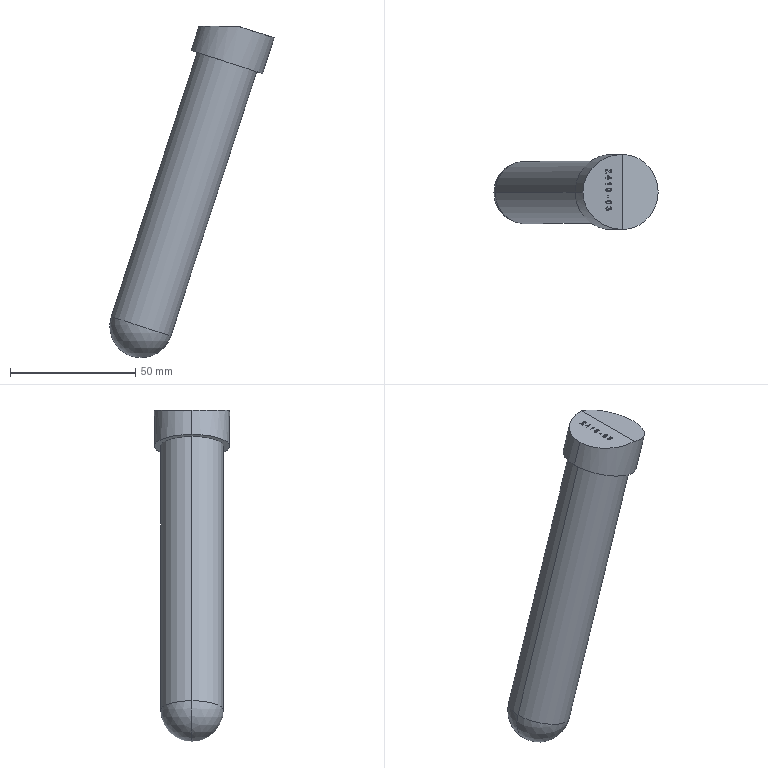Part | Creo | 1 solid | 128 faces | box 65.669 x 30 x 132.389 mm | volume 68469 mm3 | other 79 | plane 42 | cylinder 5 | sphere 2 | commonest cylinder face diameters 25 x2 30 x2 30.591 x1